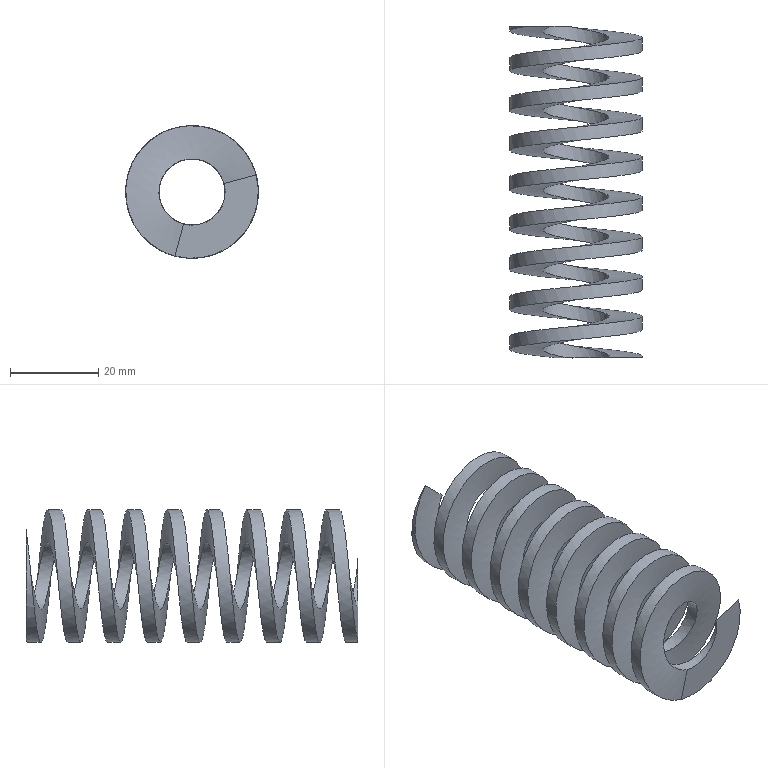Part | NX | features solid 2 | 1 solid | 6 faces | box 30.001 x 75 x 30.001 mm | volume 13165 mm3 | plane 2 | spline 2 | cylinder 2 | commonest cylinder face diameters 15 x1 30 x1